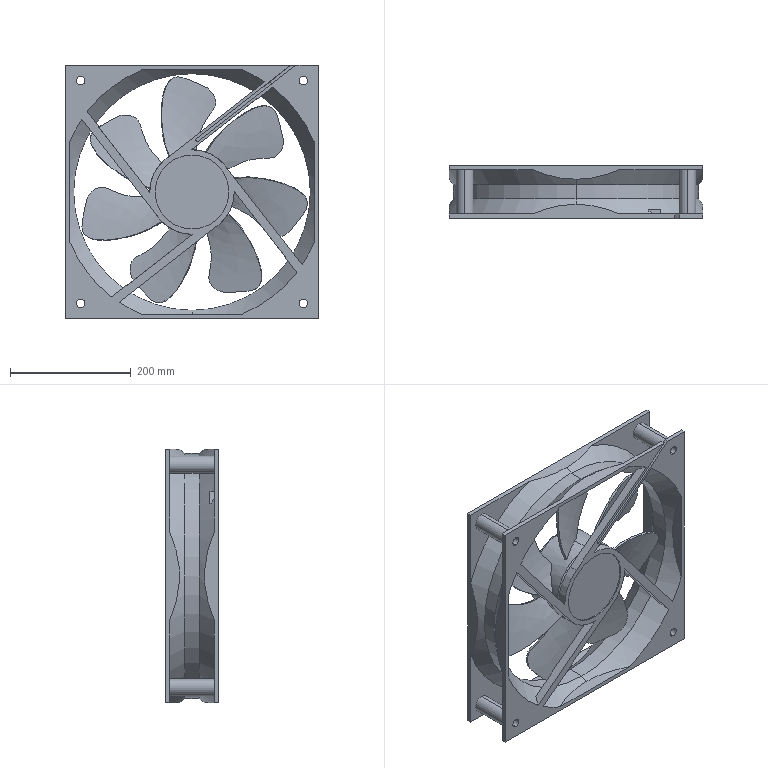Part | SolidWorks | features BaseBody 2, CombineBodies 1, Scale 1 | 1 solid | 132 faces | box 420 x 87.5 x 420 mm | volume 2233634 mm3 | plane 62 | cylinder 37 | spline 25 | cone 8 | commonest cylinder face diameters 28 x10 14 x8 140 x7 4.962 x2 17.5 x2 122.5 x2